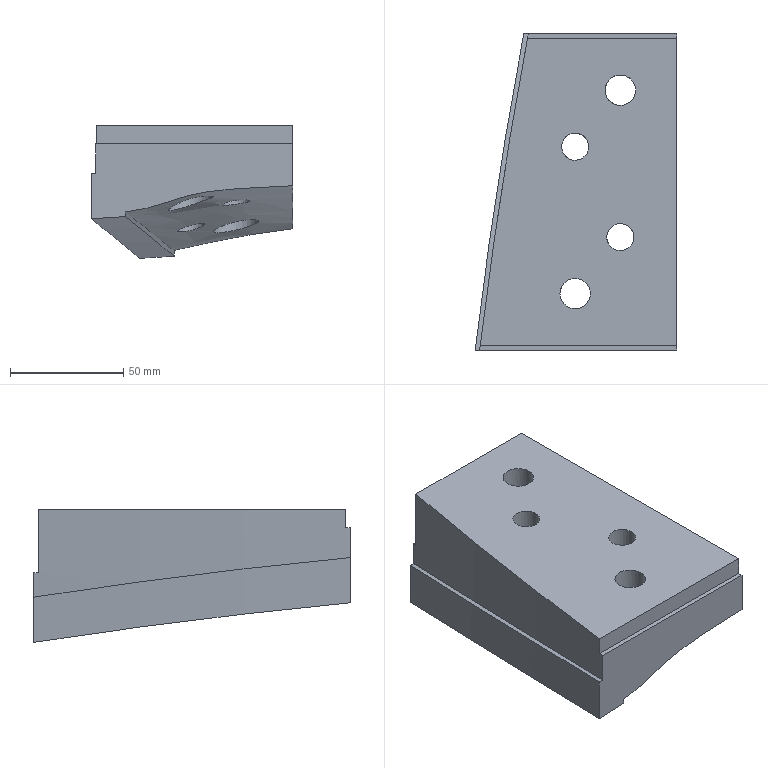Part | NX | features solid 2 | 1 solid | 22 faces | box 89.253 x 140 x 58.721 mm | volume 411184 mm3 | plane 9 | spline 7 | cylinder 6 | commonest cylinder face diameters 12 x2 13.5 x2 20 x2
STEP:
#1=CARTESIAN_POINT('',(-500.628,262.08,-55.133));
#2=VERTEX_POINT('',#1);
#3=CARTESIAN_POINT('',(-497.722,266.082,-55.166));
#4=CARTESIAN_POINT('',(-501.258,262.297,-55.273));
#5=CARTESIAN_POINT('',(-501.012,257.208,-54.545));
#6=CARTESIAN_POINT('',(-497.395,253.818,-53.31));
#7=CARTESIAN_POINT('',(-492.297,253.905,-52.638));
#8=CARTESIAN_POINT('',(-488.756,257.682,-52.752));
#9=CARTESIAN_POINT('',(-488.96,262.753,-53.541));
#10=CARTESIAN_POINT('',(-492.631,266.204,-54.446));
#11=CARTESIAN_POINT('',(-497.722,266.082,-55.166));
#12=CARTESIAN_POINT('',(-501.258,262.297,-55.273));
#13=CARTESIAN_POINT('',(-501.012,257.208,-54.545));
#14=B_SPLINE_CURVE_WITH_KNOTS('',3,(#3,#4,#5,#6,#7,#8,#9,#10,#11,#12,#13),.UNSPECIFIED.,.T.,.F.,(1,1,1,1,1,1,1,1,1,1,1,1,1,1,1),(-0.01422,-0.009479,-0.00474,0.,0.00474,0.009479,0.01422,0.01896,0.0237,0.02844,0.03318,0.03792,0.04266,0.0474,0.05214),.UNSPECIFIED.);
#15=EDGE_CURVE('',#2,#2,#14,.T.);
#16=ORIENTED_EDGE('',*,*,#15,.T.);
#17=EDGE_LOOP('',(#16));
#18=FACE_BOUND('',#17,.T.);
#19=CARTESIAN_POINT('',(-524.868,233.378,-57.001));
#20=VERTEX_POINT('',#19);
#21=CARTESIAN_POINT('',(-523.703,229.59,-56.004));
#22=CARTESIAN_POINT('',(-525.128,233.316,-57.091));
#23=CARTESIAN_POINT('',(-524.989,237.412,-57.638));
#24=CARTESIAN_POINT('',(-523.231,241.148,-57.522));
#25=CARTESIAN_POINT('',(-520.2,243.845,-56.775));
#26=CARTESIAN_POINT('',(-515.217,245.579,-55.254));
#27=CARTESIAN_POINT('',(-509.957,244.317,-53.316));
#28=CARTESIAN_POINT('',(-506.29,240.431,-52.099));
#29=CARTESIAN_POINT('',(-504.368,235.344,-51.314));
#30=CARTESIAN_POINT('',(-505.755,229.711,-50.927));
#31=CARTESIAN_POINT('',(-509.906,226.077,-51.117));
#32=CARTESIAN_POINT('',(-513.781,224.812,-51.767));
#33=CARTESIAN_POINT('',(-517.684,225.118,-53.037));
#34=CARTESIAN_POINT('',(-521.1,226.783,-54.57));
#35=CARTESIAN_POINT('',(-523.703,229.59,-56.004));
#36=CARTESIAN_POINT('',(-525.128,233.316,-57.091));
#37=CARTESIAN_POINT('',(-524.989,237.412,-57.638));
#38=B_SPLINE_CURVE_WITH_KNOTS('',3,(#21,#22,#23,#24,#25,#26,#27,#28,#29,#30,#31,#32,#33,#34,#35,#36,#37),.UNSPECIFIED.,.T.,.F.,(1,1,1,1,1,1,1,1,1,1,1,1,1,1,1,1,1,1,1,1,1),(-0.01206,-0.008041,-0.004021,0.,0.004021,0.008041,0.01206,0.01608,0.02412,0.02814,0.03216,0.04021,0.04423,0.04825,0.05227,0.05629,0.06031,0.06433,0.06835,0.07237,0.07639),.UNSPECIFIED.);
#39=EDGE_CURVE('',#20,#20,#38,.T.);
#40=ORIENTED_EDGE('',*,*,#39,.F.);
#41=EDGE_LOOP('',(#40));
#42=FACE_BOUND('',#41,.T.);
#43=CARTESIAN_POINT('',(-470.,210.,-46.611));
#44=VERTEX_POINT('',#43);
#45=CARTESIAN_POINT('',(-544.144,210.,-58.181));
#46=VERTEX_POINT('',#45);
#47=CARTESIAN_POINT('',(-470.,210.,-46.611));
#48=CARTESIAN_POINT('',(-473.142,210.,-46.734));
#49=CARTESIAN_POINT('',(-479.425,210.,-46.986));
#50=CARTESIAN_POINT('',(-488.844,210.,-47.464));
#51=CARTESIAN_POINT('',(-498.259,210.,-48.122));
#52=CARTESIAN_POINT('',(-507.638,210.,-49.048));
#53=CARTESIAN_POINT('',(-516.834,210.,-50.901));
#54=CARTESIAN_POINT('',(-525.787,210.,-54.007));
#55=CARTESIAN_POINT('',(-534.818,210.,-56.749));
#56=CARTESIAN_POINT('',(-541.02,210.,-57.77));
#57=CARTESIAN_POINT('',(-544.144,210.,-58.181));
#58=B_SPLINE_CURVE_WITH_KNOTS('',3,(#47,#48,#49,#50,#51,#52,#53,#54,#55,#56,#57),.UNSPECIFIED.,.F.,.F.,(4,1,1,1,1,1,1,1,4),(0.01237,0.0218,0.03123,0.04067,0.0501,0.05953,0.06896,0.07839,0.08783),.UNSPECIFIED.);
#59=EDGE_CURVE('',#44,#46,#58,.T.);
#60=ORIENTED_EDGE('',*,*,#59,.T.);
#61=CARTESIAN_POINT('',(-522.477,350.,-75.15));
#62=VERTEX_POINT('',#61);
#63=CARTESIAN_POINT('',(-544.144,210.,-58.181));
#64=CARTESIAN_POINT('',(-543.432,215.848,-59.019));
#65=CARTESIAN_POINT('',(-542.324,224.666,-59.797));
#66=CARTESIAN_POINT('',(-540.78,236.384,-61.12));
#67=CARTESIAN_POINT('',(-539.587,245.171,-62.09));
#68=CARTESIAN_POINT('',(-538.35,254.006,-62.555));
#69=CARTESIAN_POINT('',(-537.086,262.775,-63.591));
#70=CARTESIAN_POINT('',(-535.786,271.544,-64.601));
#71=CARTESIAN_POINT('',(-534.006,283.217,-66.034));
#72=CARTESIAN_POINT('',(-531.695,297.769,-68.007));
#73=CARTESIAN_POINT('',(-529.266,312.289,-70.077));
#74=CARTESIAN_POINT('',(-527.249,323.891,-71.737));
#75=CARTESIAN_POINT('',(-525.696,332.607,-72.823));
#76=CARTESIAN_POINT('',(-524.122,341.235,-74.542));
#77=CARTESIAN_POINT('',(-523.028,347.088,-74.878));
#78=CARTESIAN_POINT('',(-522.477,350.,-75.15));
#79=B_SPLINE_CURVE_WITH_KNOTS('',3,(#63,#64,#65,#66,#67,#68,#69,#70,#71,#72,#73,#74,#75,#76,#77,#78),.UNSPECIFIED.,.F.,.F.,(4,1,1,1,1,1,1,1,1,1,1,1,1,4),(0.1259,0.1438,0.1527,0.1616,0.1705,0.1795,0.1884,0.1973,0.2151,0.233,0.2419,0.2508,0.2597,0.2686),.UNSPECIFIED.);
#80=EDGE_CURVE('',#46,#62,#79,.T.);
#81=ORIENTED_EDGE('',*,*,#80,.T.);
#82=CARTESIAN_POINT('',(-470.,350.,-65.615));
#83=VERTEX_POINT('',#82);
#84=CARTESIAN_POINT('',(-470.,350.,-65.615));
#85=CARTESIAN_POINT('',(-478.849,350.,-66.593));
#86=CARTESIAN_POINT('',(-492.017,350.,-68.687));
#87=CARTESIAN_POINT('',(-509.435,350.,-72.287));
#88=CARTESIAN_POINT('',(-518.119,350.,-74.296));
#89=CARTESIAN_POINT('',(-522.477,350.,-75.15));
#90=B_SPLINE_CURVE_WITH_KNOTS('',3,(#84,#85,#86,#87,#88,#89),.UNSPECIFIED.,.F.,.F.,(4,1,1,4),(0.,0.02666,0.04,0.05333),.UNSPECIFIED.);
#91=EDGE_CURVE('',#83,#62,#90,.T.);
#92=ORIENTED_EDGE('',*,*,#91,.F.);
#93=CARTESIAN_POINT('',(-470.,210.,-46.611));
#94=CARTESIAN_POINT('',(-470.,212.915,-47.055));
#95=CARTESIAN_POINT('',(-470.,218.761,-47.767));
#96=CARTESIAN_POINT('',(-470.,227.581,-48.329));
#97=CARTESIAN_POINT('',(-470.,236.357,-49.332));
#98=CARTESIAN_POINT('',(-470.,245.098,-50.696));
#99=CARTESIAN_POINT('',(-470.,253.942,-51.01));
#100=CARTESIAN_POINT('',(-470.,262.68,-52.403));
#101=CARTESIAN_POINT('',(-470.,271.448,-53.491));
#102=CARTESIAN_POINT('',(-470.,283.129,-55.005));
#103=CARTESIAN_POINT('',(-470.,294.811,-56.513));
#104=CARTESIAN_POINT('',(-470.,306.491,-58.03));
#105=CARTESIAN_POINT('',(-470.,315.253,-59.159));
#106=CARTESIAN_POINT('',(-470.,324.013,-60.298));
#107=CARTESIAN_POINT('',(-470.,331.232,-61.771));
#108=CARTESIAN_POINT('',(-470.,337.094,-62.392));
#109=CARTESIAN_POINT('',(-470.,342.9,-63.373));
#110=CARTESIAN_POINT('',(-470.,347.148,-64.793));
#111=CARTESIAN_POINT('',(-470.,350.,-65.615));
#112=B_SPLINE_CURVE_WITH_KNOTS('',3,(#93,#94,#95,#96,#97,#98,#99,#100,#101,#102,#103,#104,#105,#106,#107,#108,#109,#110,#111),.UNSPECIFIED.,.F.,.F.,(4,1,1,1,1,1,1,1,1,1,1,1,1,1,1,1,4),(0.1254,0.1343,0.1431,0.152,0.1608,0.1696,0.1785,0.1873,0.1962,0.2138,0.2227,0.2315,0.2403,0.2492,0.2536,0.258,0.2669),.UNSPECIFIED.);
#113=EDGE_CURVE('',#44,#83,#112,.T.);
#114=ORIENTED_EDGE('',*,*,#113,.F.);
#115=EDGE_LOOP('',(#60,#81,#92,#114));
#116=FACE_BOUND('',#115,.T.);
#117=CARTESIAN_POINT('',(-520.662,301.985,-66.934));
#118=VERTEX_POINT('',#117);
#119=CARTESIAN_POINT('',(-517.742,306.086,-67.045));
#120=CARTESIAN_POINT('',(-521.321,302.19,-67.104));
#121=CARTESIAN_POINT('',(-520.946,297.06,-66.142));
#122=CARTESIAN_POINT('',(-517.246,293.781,-64.691));
#123=CARTESIAN_POINT('',(-512.236,293.932,-63.34));
#124=CARTESIAN_POINT('',(-508.673,297.826,-63.049));
#125=CARTESIAN_POINT('',(-509.068,302.943,-64.101));
#126=CARTESIAN_POINT('',(-512.703,306.194,-65.747));
#127=CARTESIAN_POINT('',(-517.742,306.086,-67.045));
#128=CARTESIAN_POINT('',(-521.321,302.19,-67.104));
#129=CARTESIAN_POINT('',(-520.946,297.06,-66.142));
#130=B_SPLINE_CURVE_WITH_KNOTS('',3,(#119,#120,#121,#122,#123,#124,#125,#126,#127,#128,#129),.UNSPECIFIED.,.T.,.F.,(1,1,1,1,1,1,1,1,1,1,1,1,1,1,1),(-0.01442,-0.009613,-0.004806,0.,0.004806,0.009613,0.01442,0.01923,0.02403,0.02884,0.03364,0.03845,0.04326,0.04806,0.05287),.UNSPECIFIED.);
#131=EDGE_CURVE('',#118,#118,#130,.T.);
#132=ORIENTED_EDGE('',*,*,#131,.T.);
#133=EDGE_LOOP('',(#132));
#134=FACE_BOUND('',#133,.T.);
#135=CARTESIAN_POINT('',(-485.071,326.186,-62.407));
#136=VERTEX_POINT('',#135);
#137=CARTESIAN_POINT('',(-488.149,333.648,-64.251));
#138=CARTESIAN_POINT('',(-483.99,326.362,-62.241));
#139=CARTESIAN_POINT('',(-486.314,318.019,-61.23));
#140=CARTESIAN_POINT('',(-494.001,313.958,-61.995));
#141=CARTESIAN_POINT('',(-501.898,316.427,-64.409));
#142=CARTESIAN_POINT('',(-505.271,322.343,-66.559));
#143=CARTESIAN_POINT('',(-504.897,327.749,-67.252));
#144=CARTESIAN_POINT('',(-503.038,331.396,-67.351));
#145=CARTESIAN_POINT('',(-499.902,334.024,-67.137));
#146=CARTESIAN_POINT('',(-494.738,335.605,-66.229));
#147=CARTESIAN_POINT('',(-488.149,333.648,-64.251));
#148=CARTESIAN_POINT('',(-483.99,326.362,-62.241));
#149=CARTESIAN_POINT('',(-486.314,318.019,-61.23));
#150=B_SPLINE_CURVE_WITH_KNOTS('',3,(#137,#138,#139,#140,#141,#142,#143,#144,#145,#146,#147,#148,#149),.UNSPECIFIED.,.T.,.F.,(1,1,1,1,1,1,1,1,1,1,1,1,1,1,1,1,1),(-0.01996,-0.01597,-0.007984,0.,0.007984,0.01597,0.02395,0.03194,0.03593,0.03992,0.04391,0.0479,0.05589,0.06387,0.07186,0.07984,0.08782),.UNSPECIFIED.);
#151=EDGE_CURVE('',#136,#136,#150,.T.);
#152=ORIENTED_EDGE('',*,*,#151,.F.);
#153=EDGE_LOOP('',(#152));
#154=FACE_BOUND('',#153,.T.);
#155=CARTESIAN_POINT('',(-449.856,350.,-63.928));
#156=CARTESIAN_POINT('',(-450.513,346.762,-63.155));
#157=CARTESIAN_POINT('',(-451.724,340.897,-61.568));
#158=CARTESIAN_POINT('',(-453.043,332.345,-61.292));
#159=CARTESIAN_POINT('',(-454.751,323.079,-59.482));
#160=CARTESIAN_POINT('',(-456.154,313.774,-58.463));
#161=CARTESIAN_POINT('',(-457.767,303.143,-57.153));
#162=CARTESIAN_POINT('',(-459.124,293.837,-56.036));
#163=CARTESIAN_POINT('',(-460.633,283.202,-54.741));
#164=CARTESIAN_POINT('',(-461.944,273.894,-53.558));
#165=CARTESIAN_POINT('',(-463.37,263.256,-52.318));
#166=CARTESIAN_POINT('',(-464.678,253.944,-50.886));
#167=CARTESIAN_POINT('',(-465.814,243.308,-50.34));
#168=CARTESIAN_POINT('',(-467.008,233.989,-48.769));
#169=CARTESIAN_POINT('',(-468.149,223.335,-47.963));
#170=CARTESIAN_POINT('',(-468.958,215.772,-47.418));
#171=CARTESIAN_POINT('',(-469.452,210.889,-46.724));
#172=CARTESIAN_POINT('',(-469.542,210.,-46.593));
#173=CARTESIAN_POINT('',(-458.824,350.,-64.479));
#174=CARTESIAN_POINT('',(-459.498,346.762,-63.609));
#175=CARTESIAN_POINT('',(-460.741,340.897,-61.784));
#176=CARTESIAN_POINT('',(-462.105,332.345,-61.543));
#177=CARTESIAN_POINT('',(-463.848,323.079,-59.715));
#178=CARTESIAN_POINT('',(-465.277,313.774,-58.704));
#179=CARTESIAN_POINT('',(-466.92,303.143,-57.386));
#180=CARTESIAN_POINT('',(-468.301,293.837,-56.271));
#181=CARTESIAN_POINT('',(-469.838,283.202,-54.976));
#182=CARTESIAN_POINT('',(-471.174,273.894,-53.77));
#183=CARTESIAN_POINT('',(-472.622,263.256,-52.566));
#184=CARTESIAN_POINT('',(-473.97,253.944,-51.01));
#185=CARTESIAN_POINT('',(-475.086,243.308,-50.852));
#186=CARTESIAN_POINT('',(-476.315,233.989,-49.173));
#187=CARTESIAN_POINT('',(-477.474,223.335,-48.448));
#188=CARTESIAN_POINT('',(-478.287,215.772,-47.966));
#189=CARTESIAN_POINT('',(-478.816,210.889,-47.117));
#190=CARTESIAN_POINT('',(-478.912,210.,-46.959));
#191=CARTESIAN_POINT('',(-473.435,350.,-65.726));
#192=CARTESIAN_POINT('',(-474.128,346.762,-64.77));
#193=CARTESIAN_POINT('',(-475.402,340.897,-62.756));
#194=CARTESIAN_POINT('',(-476.899,332.345,-62.044));
#195=CARTESIAN_POINT('',(-478.685,323.079,-60.267));
#196=CARTESIAN_POINT('',(-480.159,313.774,-59.241));
#197=CARTESIAN_POINT('',(-481.852,303.143,-57.9));
#198=CARTESIAN_POINT('',(-483.273,293.837,-56.782));
#199=CARTESIAN_POINT('',(-484.856,283.202,-55.473));
#200=CARTESIAN_POINT('',(-486.235,273.894,-54.23));
#201=CARTESIAN_POINT('',(-487.725,263.256,-53.066));
#202=CARTESIAN_POINT('',(-489.113,253.944,-51.363));
#203=CARTESIAN_POINT('',(-490.278,243.308,-51.691));
#204=CARTESIAN_POINT('',(-491.533,233.989,-49.951));
#205=CARTESIAN_POINT('',(-492.732,223.335,-49.263));
#206=CARTESIAN_POINT('',(-493.563,215.772,-48.871));
#207=CARTESIAN_POINT('',(-494.125,210.889,-47.791));
#208=CARTESIAN_POINT('',(-494.227,210.,-47.592));
#209=CARTESIAN_POINT('',(-493.528,350.,-69.004));
#210=CARTESIAN_POINT('',(-494.177,346.762,-68.601));
#211=CARTESIAN_POINT('',(-495.352,340.897,-67.906));
#212=CARTESIAN_POINT('',(-496.974,332.345,-65.437));
#213=CARTESIAN_POINT('',(-498.685,323.079,-64.394));
#214=CARTESIAN_POINT('',(-500.264,313.774,-63.172));
#215=CARTESIAN_POINT('',(-502.032,303.143,-61.81));
#216=CARTESIAN_POINT('',(-503.541,293.837,-60.561));
#217=CARTESIAN_POINT('',(-505.215,283.202,-59.125));
#218=CARTESIAN_POINT('',(-506.619,273.894,-57.989));
#219=CARTESIAN_POINT('',(-508.284,263.256,-56.294));
#220=CARTESIAN_POINT('',(-509.365,253.944,-56.111));
#221=CARTESIAN_POINT('',(-511.739,243.308,-51.7));
#222=CARTESIAN_POINT('',(-512.661,233.989,-51.783));
#223=CARTESIAN_POINT('',(-513.992,223.335,-50.536));
#224=CARTESIAN_POINT('',(-515.05,215.772,-49.254));
#225=CARTESIAN_POINT('',(-515.27,210.889,-49.774));
#226=CARTESIAN_POINT('',(-515.308,210.,-49.876));
#227=CARTESIAN_POINT('',(-508.923,350.,-72.168));
#228=CARTESIAN_POINT('',(-509.556,346.762,-72.055));
#229=CARTESIAN_POINT('',(-510.683,340.897,-72.06));
#230=CARTESIAN_POINT('',(-512.084,332.345,-70.049));
#231=CARTESIAN_POINT('',(-513.723,323.079,-69.619));
#232=CARTESIAN_POINT('',(-515.396,313.774,-68.202));
#233=CARTESIAN_POINT('',(-517.233,303.143,-66.813));
#234=CARTESIAN_POINT('',(-518.821,293.837,-65.444));
#235=CARTESIAN_POINT('',(-520.563,283.202,-63.955));
#236=CARTESIAN_POINT('',(-522.016,273.894,-62.801));
#237=CARTESIAN_POINT('',(-523.686,263.256,-61.26));
#238=CARTESIAN_POINT('',(-525.022,253.944,-60.29));
#239=CARTESIAN_POINT('',(-526.333,243.308,-59.951));
#240=CARTESIAN_POINT('',(-527.611,233.989,-58.843));
#241=CARTESIAN_POINT('',(-529.001,223.335,-57.605));
#242=CARTESIAN_POINT('',(-529.929,215.772,-56.934));
#243=CARTESIAN_POINT('',(-530.518,210.889,-56.17));
#244=CARTESIAN_POINT('',(-530.626,210.,-56.028));
#245=CARTESIAN_POINT('',(-518.692,350.,-74.418));
#246=CARTESIAN_POINT('',(-519.336,346.762,-74.182));
#247=CARTESIAN_POINT('',(-520.478,340.897,-73.967));
#248=CARTESIAN_POINT('',(-521.951,332.345,-72.164));
#249=CARTESIAN_POINT('',(-523.639,323.079,-71.205));
#250=CARTESIAN_POINT('',(-525.351,313.774,-69.84));
#251=CARTESIAN_POINT('',(-527.235,303.143,-68.345));
#252=CARTESIAN_POINT('',(-528.845,293.837,-67.064));
#253=CARTESIAN_POINT('',(-530.615,283.202,-65.615));
#254=CARTESIAN_POINT('',(-532.096,273.894,-64.454));
#255=CARTESIAN_POINT('',(-533.76,263.256,-63.183));
#256=CARTESIAN_POINT('',(-535.149,253.944,-62.094));
#257=CARTESIAN_POINT('',(-536.435,243.308,-61.647));
#258=CARTESIAN_POINT('',(-537.767,233.989,-60.473));
#259=CARTESIAN_POINT('',(-539.173,223.335,-59.346));
#260=CARTESIAN_POINT('',(-540.107,215.772,-58.653));
#261=CARTESIAN_POINT('',(-540.738,210.889,-57.918));
#262=CARTESIAN_POINT('',(-540.853,210.,-57.782));
#263=CARTESIAN_POINT('',(-522.907,350.,-75.234));
#264=CARTESIAN_POINT('',(-523.558,346.762,-74.932));
#265=CARTESIAN_POINT('',(-524.71,340.897,-74.582));
#266=CARTESIAN_POINT('',(-526.228,332.345,-72.867));
#267=CARTESIAN_POINT('',(-527.941,323.079,-71.701));
#268=CARTESIAN_POINT('',(-529.668,313.774,-70.369));
#269=CARTESIAN_POINT('',(-531.571,303.143,-68.846));
#270=CARTESIAN_POINT('',(-533.189,293.837,-67.602));
#271=CARTESIAN_POINT('',(-534.971,283.202,-66.172));
#272=CARTESIAN_POINT('',(-536.463,273.894,-65.007));
#273=CARTESIAN_POINT('',(-538.128,263.256,-63.818));
#274=CARTESIAN_POINT('',(-539.531,253.944,-62.697));
#275=CARTESIAN_POINT('',(-540.854,243.308,-62.069));
#276=CARTESIAN_POINT('',(-542.194,233.989,-60.923));
#277=CARTESIAN_POINT('',(-543.607,223.335,-59.841));
#278=CARTESIAN_POINT('',(-544.55,215.772,-59.117));
#279=CARTESIAN_POINT('',(-545.183,210.889,-58.451));
#280=CARTESIAN_POINT('',(-545.298,210.,-58.327));
#281=B_SPLINE_SURFACE_WITH_KNOTS('',3,3,((#155,#156,#157,#158,#159,#160,#161,#162,#163,#164,#165,#166,#167,#168,#169,#170,#171,#172),(#173,#174,#175,#176,#177,#178,#179,#180,#181,#182,#183,#184,#185,#186,#187,#188,#189,#190),(#191,#192,#193,#194,#195,#196,#197,#198,#199,#200,#201,#202,#203,#204,#205,#206,#207,#208),(#209,#210,#211,#212,#213,#214,#215,#216,#217,#218,#219,#220,#221,#222,#223,#224,#225,#226),(#227,#228,#229,#230,#231,#232,#233,#234,#235,#236,#237,#238,#239,#240,#241,#242,#243,#244),(#245,#246,#247,#248,#249,#250,#251,#252,#253,#254,#255,#256,#257,#258,#259,#260,#261,#262),(#263,#264,#265,#266,#267,#268,#269,#270,#271,#272,#273,#274,#275,#276,#277,#278,#279,#280)),.UNSPECIFIED.,.F.,.F.,.F.,(4,1,1,1,4),(4,1,1,1,1,1,1,1,1,1,1,1,1,1,1,4),(0.9128,0.9375,0.9531,0.9688,0.9806),(0.2465,0.2656,0.2812,0.2969,0.3203,0.3359,0.3594,0.375,0.3984,0.4141,0.4375,0.4531,0.4766,0.4922,0.5156,0.5208),.UNSPECIFIED.);
#282=ADVANCED_FACE('',(#18,#42,#116,#134,#154),#281,.F.);
#283=CARTESIAN_POINT('',(-470.,348.,-48.));
#284=VERTEX_POINT('',#283);
#285=CARTESIAN_POINT('',(-536.081,348.,-48.));
#286=VERTEX_POINT('',#285);
#287=CARTESIAN_POINT('',(-470.,348.,-48.));
#288=DIRECTION('',(1.,0.,0.));
#289=VECTOR('',#288,1000.);
#290=LINE('',#287,#289);
#291=EDGE_CURVE('',#284,#286,#290,.F.);
#292=ORIENTED_EDGE('',*,*,#291,.F.);
#293=CARTESIAN_POINT('',(-470.,350.,-48.));
#294=VERTEX_POINT('',#293);
#295=CARTESIAN_POINT('',(-470.,350.,-48.));
#296=DIRECTION('',(0.,1.,0.));
#297=VECTOR('',#296,1000.);
#298=LINE('',#295,#297);
#299=EDGE_CURVE('',#294,#284,#298,.F.);
#300=ORIENTED_EDGE('',*,*,#299,.F.);
#301=CARTESIAN_POINT('',(-535.705,350.,-48.));
#302=VERTEX_POINT('',#301);
#303=CARTESIAN_POINT('',(-470.,350.,-48.));
#304=DIRECTION('',(1.,0.,0.));
#305=VECTOR('',#304,1000.);
#306=LINE('',#303,#305);
#307=EDGE_CURVE('',#294,#302,#306,.F.);
#308=ORIENTED_EDGE('',*,*,#307,.T.);
#309=CARTESIAN_POINT('',(-536.081,348.,-48.));
#310=CARTESIAN_POINT('',(-535.956,348.667,-48.));
#311=CARTESIAN_POINT('',(-535.831,349.333,-48.));
#312=CARTESIAN_POINT('',(-535.705,350.,-48.));
#313=B_SPLINE_CURVE_WITH_KNOTS('',3,(#309,#310,#311,#312),.UNSPECIFIED.,.F.,.F.,(4,4),(0.01222,0.01426),.UNSPECIFIED.);
#314=EDGE_CURVE('',#302,#286,#313,.F.);
#315=ORIENTED_EDGE('',*,*,#314,.T.);
#316=EDGE_LOOP('',(#292,#300,#308,#315));
#317=FACE_BOUND('',#316,.T.);
#318=CARTESIAN_POINT('',(-470.,350.,-48.));
#319=DIRECTION('',(0.,0.,1.));
#320=DIRECTION('',(1.,0.,0.));
#321=AXIS2_PLACEMENT_3D('',#318,#319,#320);
#322=PLANE('',#321);
#323=ADVANCED_FACE('',(#317),#322,.T.);
#324=CARTESIAN_POINT('',(-535.705,350.,-58.778));
#325=VERTEX_POINT('',#324);
#326=CARTESIAN_POINT('',(-535.705,350.,-23.36));
#327=DIRECTION('',(0.,0.,1.));
#328=VECTOR('',#327,1000.);
#329=LINE('',#326,#328);
#330=EDGE_CURVE('',#325,#302,#329,.T.);
#331=ORIENTED_EDGE('',*,*,#330,.T.);
#332=ORIENTED_EDGE('',*,*,#307,.F.);
#333=CARTESIAN_POINT('',(-470.,350.,-40.306));
#334=DIRECTION('',(0.,0.,-1.));
#335=VECTOR('',#334,1000.);
#336=LINE('',#333,#335);
#337=EDGE_CURVE('',#83,#294,#336,.F.);
#338=ORIENTED_EDGE('',*,*,#337,.F.);
#339=ORIENTED_EDGE('',*,*,#91,.T.);
#340=CARTESIAN_POINT('',(-522.477,350.,-77.768));
#341=VERTEX_POINT('',#340);
#342=CARTESIAN_POINT('',(-522.477,350.,-46.));
#343=DIRECTION('',(0.,0.,1.));
#344=VECTOR('',#343,1000.);
#345=LINE('',#342,#344);
#346=EDGE_CURVE('',#341,#62,#345,.T.);
#347=ORIENTED_EDGE('',*,*,#346,.F.);
#348=CARTESIAN_POINT('',(-537.74,350.,-78.721));
#349=VERTEX_POINT('',#348);
#350=CARTESIAN_POINT('',(-537.74,350.,-78.721));
#351=CARTESIAN_POINT('',(-532.653,350.,-78.396));
#352=CARTESIAN_POINT('',(-527.565,350.,-78.079));
#353=CARTESIAN_POINT('',(-522.477,350.,-77.768));
#354=B_SPLINE_CURVE_WITH_KNOTS('',3,(#350,#351,#352,#353),.UNSPECIFIED.,.F.,.F.,(4,4),(0.03478,0.05008),.UNSPECIFIED.);
#355=EDGE_CURVE('',#349,#341,#354,.T.);
#356=ORIENTED_EDGE('',*,*,#355,.F.);
#357=CARTESIAN_POINT('',(-537.74,350.,-58.721));
#358=VERTEX_POINT('',#357);
#359=CARTESIAN_POINT('',(-537.74,350.,-41.428));
#360=DIRECTION('',(0.,0.,1.));
#361=VECTOR('',#360,1000.);
#362=LINE('',#359,#361);
#363=EDGE_CURVE('',#358,#349,#362,.F.);
#364=ORIENTED_EDGE('',*,*,#363,.F.);
#365=CARTESIAN_POINT('',(-535.705,350.,-58.778));
#366=CARTESIAN_POINT('',(-536.384,350.,-58.759));
#367=CARTESIAN_POINT('',(-537.062,350.,-58.74));
#368=CARTESIAN_POINT('',(-537.74,350.,-58.721));
#369=B_SPLINE_CURVE_WITH_KNOTS('',3,(#365,#366,#367,#368),.UNSPECIFIED.,.F.,.F.,(4,4),(0.008143,0.01018),.UNSPECIFIED.);
#370=EDGE_CURVE('',#358,#325,#369,.F.);
#371=ORIENTED_EDGE('',*,*,#370,.T.);
#372=EDGE_LOOP('',(#331,#332,#338,#339,#347,#356,#364,#371));
#373=FACE_BOUND('',#372,.T.);
#374=CARTESIAN_POINT('',(440.921,350.,-40.306));
#375=DIRECTION('',(0.,1.,0.));
#376=DIRECTION('',(0.,0.,1.));
#377=AXIS2_PLACEMENT_3D('',#374,#375,#376);
#378=PLANE('',#377);
#379=ADVANCED_FACE('',(#373),#378,.T.);
#380=CARTESIAN_POINT('',(-470.,348.,-20.));
#381=VERTEX_POINT('',#380);
#382=CARTESIAN_POINT('',(-470.,348.,12.));
#383=DIRECTION('',(0.,0.,1.));
#384=VECTOR('',#383,1000.);
#385=LINE('',#382,#384);
#386=EDGE_CURVE('',#381,#284,#385,.F.);
#387=ORIENTED_EDGE('',*,*,#386,.T.);
#388=ORIENTED_EDGE('',*,*,#291,.T.);
#389=CARTESIAN_POINT('',(-536.081,348.,-20.));
#390=VERTEX_POINT('',#389);
#391=CARTESIAN_POINT('',(-536.081,348.,-18.));
#392=DIRECTION('',(0.,0.,1.));
#393=VECTOR('',#392,1000.);
#394=LINE('',#391,#393);
#395=EDGE_CURVE('',#390,#286,#394,.F.);
#396=ORIENTED_EDGE('',*,*,#395,.F.);
#397=CARTESIAN_POINT('',(-470.,348.,-20.));
#398=DIRECTION('',(-1.,0.,0.));
#399=VECTOR('',#398,1000.);
#400=LINE('',#397,#399);
#401=EDGE_CURVE('',#381,#390,#400,.T.);
#402=ORIENTED_EDGE('',*,*,#401,.F.);
#403=EDGE_LOOP('',(#387,#388,#396,#402));
#404=FACE_BOUND('',#403,.T.);
#405=CARTESIAN_POINT('',(-470.,348.,12.));
#406=DIRECTION('',(0.,1.,0.));
#407=DIRECTION('',(-1.,0.,0.));
#408=AXIS2_PLACEMENT_3D('',#405,#406,#407);
#409=PLANE('',#408);
#410=ADVANCED_FACE('',(#404),#409,.T.);
#411=CARTESIAN_POINT('',(-544.144,210.,-60.227));
#412=VERTEX_POINT('',#411);
#413=CARTESIAN_POINT('',(-544.144,210.,-60.227));
#414=CARTESIAN_POINT('',(-538.417,257.027,-64.777));
#415=CARTESIAN_POINT('',(-531.226,303.745,-70.657));
#416=CARTESIAN_POINT('',(-522.477,350.,-77.768));
#417=B_SPLINE_CURVE_WITH_KNOTS('',3,(#413,#414,#415,#416),.UNSPECIFIED.,.F.,.F.,(4,4),(0.1259,0.2687),.UNSPECIFIED.);
#418=EDGE_CURVE('',#412,#341,#417,.T.);
#419=ORIENTED_EDGE('',*,*,#418,.T.);
#420=ORIENTED_EDGE('',*,*,#346,.T.);
#421=ORIENTED_EDGE('',*,*,#80,.F.);
#422=CARTESIAN_POINT('',(-544.144,210.,-63.127));
#423=DIRECTION('',(0.,0.,1.));
#424=VECTOR('',#423,1000.);
#425=LINE('',#422,#424);
#426=EDGE_CURVE('',#412,#46,#425,.T.);
#427=ORIENTED_EDGE('',*,*,#426,.F.);
#428=EDGE_LOOP('',(#419,#420,#421,#427));
#429=FACE_BOUND('',#428,.T.);
#430=CARTESIAN_POINT('',(-522.477,350.,-77.886));
#431=CARTESIAN_POINT('',(-522.477,350.,-58.063));
#432=CARTESIAN_POINT('',(-524.645,338.539,-77.886));
#433=CARTESIAN_POINT('',(-524.645,338.539,-58.063));
#434=CARTESIAN_POINT('',(-528.8,315.507,-77.886));
#435=CARTESIAN_POINT('',(-528.8,315.507,-58.063));
#436=CARTESIAN_POINT('',(-534.491,280.641,-77.886));
#437=CARTESIAN_POINT('',(-534.491,280.641,-58.063));
#438=CARTESIAN_POINT('',(-538.785,251.287,-77.886));
#439=CARTESIAN_POINT('',(-538.785,251.287,-58.063));
#440=CARTESIAN_POINT('',(-541.548,230.648,-77.886));
#441=CARTESIAN_POINT('',(-541.548,230.648,-58.063));
#442=CARTESIAN_POINT('',(-543.069,218.732,-77.886));
#443=CARTESIAN_POINT('',(-543.069,218.732,-58.063));
#444=CARTESIAN_POINT('',(-543.788,212.925,-77.886));
#445=CARTESIAN_POINT('',(-543.788,212.925,-58.063));
#446=CARTESIAN_POINT('',(-544.144,210.,-77.886));
#447=CARTESIAN_POINT('',(-544.144,210.,-58.063));
#448=B_SPLINE_SURFACE_WITH_KNOTS('',3,1,((#430,#431),(#432,#433),(#434,#435),(#436,#437),(#438,#439),(#440,#441),(#442,#443),(#444,#445),(#446,#447)),.SURF_OF_LINEAR_EXTRUSION.,.F.,.F.,.F.,(4,1,1,1,1,1,4),(2,2),(0.005019,0.1372,0.2694,0.4015,0.4676,0.5007,0.5337),(0.,1.),.UNSPECIFIED.);
#449=ADVANCED_FACE('',(#429),#448,.F.);
#450=CARTESIAN_POINT('',(-557.238,210.,-41.223));
#451=VERTEX_POINT('',#450);
#452=CARTESIAN_POINT('',(-557.238,210.,-41.223));
#453=CARTESIAN_POINT('',(-551.535,257.074,-45.781));
#454=CARTESIAN_POINT('',(-544.405,303.746,-51.67));
#455=CARTESIAN_POINT('',(-535.705,350.,-58.778));
#456=B_SPLINE_CURVE_WITH_KNOTS('',3,(#452,#453,#454,#455),.UNSPECIFIED.,.F.,.F.,(4,4),(0.4694,1.001),.UNSPECIFIED.);
#457=EDGE_CURVE('',#325,#451,#456,.F.);
#458=ORIENTED_EDGE('',*,*,#457,.F.);
#459=ORIENTED_EDGE('',*,*,#370,.F.);
#460=CARTESIAN_POINT('',(-559.253,210.,-41.2));
#461=VERTEX_POINT('',#460);
#462=CARTESIAN_POINT('',(-537.74,350.,-58.721));
#463=CARTESIAN_POINT('',(-539.944,338.283,-56.922));
#464=CARTESIAN_POINT('',(-544.14,314.869,-53.494));
#465=CARTESIAN_POINT('',(-549.8,279.843,-48.863));
#466=CARTESIAN_POINT('',(-554.857,244.877,-44.737));
#467=CARTESIAN_POINT('',(-557.83,221.759,-42.336));
#468=CARTESIAN_POINT('',(-559.253,210.,-41.2));
#469=B_SPLINE_CURVE_WITH_KNOTS('',3,(#462,#463,#464,#465,#466,#467,#468),.UNSPECIFIED.,.F.,.F.,(4,1,1,1,4),(0.,0.1328,0.2657,0.3985,0.5314),.UNSPECIFIED.);
#470=EDGE_CURVE('',#358,#461,#469,.T.);
#471=ORIENTED_EDGE('',*,*,#470,.T.);
#472=CARTESIAN_POINT('',(-557.238,210.,-41.223));
#473=CARTESIAN_POINT('',(-557.91,210.,-41.215));
#474=CARTESIAN_POINT('',(-558.581,210.,-41.208));
#475=CARTESIAN_POINT('',(-559.253,210.,-41.2));
#476=B_SPLINE_CURVE_WITH_KNOTS('',3,(#472,#473,#474,#475),.UNSPECIFIED.,.F.,.F.,(4,4),(0.,0.002015),.UNSPECIFIED.);
#477=EDGE_CURVE('',#451,#461,#476,.T.);
#478=ORIENTED_EDGE('',*,*,#477,.F.);
#479=EDGE_LOOP('',(#458,#459,#471,#478));
#480=FACE_BOUND('',#479,.T.);
#481=CARTESIAN_POINT('',(-535.549,350.834,-58.906));
#482=CARTESIAN_POINT('',(-535.624,350.433,-58.844));
#483=CARTESIAN_POINT('',(-535.699,350.032,-58.782));
#484=CARTESIAN_POINT('',(-535.775,349.63,-58.721));
#485=CARTESIAN_POINT('',(-543.951,306.163,-52.041));
#486=CARTESIAN_POINT('',(-550.731,262.328,-46.45));
#487=CARTESIAN_POINT('',(-556.622,215.058,-41.716));
#488=CARTESIAN_POINT('',(-556.999,211.985,-41.414));
#489=CARTESIAN_POINT('',(-557.37,208.911,-41.118));
#490=CARTESIAN_POINT('',(-537.514,351.205,-58.906));
#491=CARTESIAN_POINT('',(-537.589,350.803,-58.844));
#492=CARTESIAN_POINT('',(-537.665,350.402,-58.782));
#493=CARTESIAN_POINT('',(-537.74,350.,-58.721));
#494=CARTESIAN_POINT('',(-545.924,306.491,-52.041));
#495=CARTESIAN_POINT('',(-552.711,262.613,-46.45));
#496=CARTESIAN_POINT('',(-558.607,215.302,-41.716));
#497=CARTESIAN_POINT('',(-558.984,212.227,-41.414));
#498=CARTESIAN_POINT('',(-559.356,209.15,-41.118));
#499=B_SPLINE_SURFACE_WITH_KNOTS('',1,3,((#481,#482,#483,#484,#485,#486,#487,#488,#489),(#490,#491,#492,#493,#494,#495,#496,#497,#498)),.RULED_SURF.,.F.,.F.,.F.,(2,2),(4,3,2,4),(0.,1.),(-0.004615,0.,0.5,0.5347),.UNSPECIFIED.);
#500=ADVANCED_FACE('',(#480),#499,.T.);
#501=ORIENTED_EDGE('',*,*,#470,.F.);
#502=ORIENTED_EDGE('',*,*,#363,.T.);
#503=CARTESIAN_POINT('',(-559.253,210.,-61.2));
#504=VERTEX_POINT('',#503);
#505=CARTESIAN_POINT('',(-537.74,350.,-78.721));
#506=CARTESIAN_POINT('',(-546.44,303.747,-71.62));
#507=CARTESIAN_POINT('',(-553.557,257.075,-65.75));
#508=CARTESIAN_POINT('',(-559.253,210.,-61.2));
#509=B_SPLINE_CURVE_WITH_KNOTS('',3,(#505,#506,#507,#508),.UNSPECIFIED.,.F.,.F.,(4,4),(0.3116,0.4563),.UNSPECIFIED.);
#510=EDGE_CURVE('',#349,#504,#509,.T.);
#511=ORIENTED_EDGE('',*,*,#510,.T.);
#512=CARTESIAN_POINT('',(-559.253,210.,-55.491));
#513=DIRECTION('',(0.,0.,1.));
#514=VECTOR('',#513,1000.);
#515=LINE('',#512,#514);
#516=EDGE_CURVE('',#461,#504,#515,.F.);
#517=ORIENTED_EDGE('',*,*,#516,.F.);
#518=EDGE_LOOP('',(#501,#502,#511,#517));
#519=FACE_BOUND('',#518,.T.);
#520=CARTESIAN_POINT('',(-559.355,209.153,-78.946));
#521=CARTESIAN_POINT('',(-559.355,209.153,-40.975));
#522=CARTESIAN_POINT('',(-553.648,256.468,-78.946));
#523=CARTESIAN_POINT('',(-553.648,256.468,-40.975));
#524=CARTESIAN_POINT('',(-546.491,303.477,-78.946));
#525=CARTESIAN_POINT('',(-546.491,303.477,-40.975));
#526=CARTESIAN_POINT('',(-537.74,350.,-78.946));
#527=CARTESIAN_POINT('',(-537.74,350.,-40.975));
#528=B_SPLINE_SURFACE_WITH_KNOTS('',3,1,((#520,#521),(#522,#523),(#524,#525),(#526,#527)),.SURF_OF_LINEAR_EXTRUSION.,.F.,.F.,.F.,(4,4),(2,2),(0.3283,0.4272),(0.,1.),.PIECEWISE_BEZIER_KNOTS.);
#529=ADVANCED_FACE('',(#519),#528,.F.);
#530=ORIENTED_EDGE('',*,*,#510,.F.);
#531=ORIENTED_EDGE('',*,*,#355,.T.);
#532=ORIENTED_EDGE('',*,*,#418,.F.);
#533=CARTESIAN_POINT('',(-559.253,210.,-61.2));
#534=CARTESIAN_POINT('',(-554.217,210.,-60.868));
#535=CARTESIAN_POINT('',(-549.18,210.,-60.544));
#536=CARTESIAN_POINT('',(-544.144,210.,-60.227));
#537=B_SPLINE_CURVE_WITH_KNOTS('',3,(#533,#534,#535,#536),.UNSPECIFIED.,.F.,.F.,(4,4),(0.01195,0.02709),.UNSPECIFIED.);
#538=EDGE_CURVE('',#504,#412,#537,.T.);
#539=ORIENTED_EDGE('',*,*,#538,.F.);
#540=EDGE_LOOP('',(#530,#531,#532,#539));
#541=FACE_BOUND('',#540,.T.);
#542=CARTESIAN_POINT('',(-559.416,351.134,-80.335));
#543=CARTESIAN_POINT('',(-547.03,351.032,-79.478));
#544=CARTESIAN_POINT('',(-534.643,350.935,-78.665));
#545=CARTESIAN_POINT('',(-522.256,350.843,-77.894));
#546=CARTESIAN_POINT('',(-559.434,303.646,-72.44));
#547=CARTESIAN_POINT('',(-547.048,303.545,-71.593));
#548=CARTESIAN_POINT('',(-534.662,303.45,-70.792));
#549=CARTESIAN_POINT('',(-522.275,303.359,-70.032));
#550=CARTESIAN_POINT('',(-559.453,256.323,-66.037));
#551=CARTESIAN_POINT('',(-547.068,256.223,-65.201));
#552=CARTESIAN_POINT('',(-534.682,256.128,-64.41));
#553=CARTESIAN_POINT('',(-522.294,256.039,-63.66));
#554=CARTESIAN_POINT('',(-559.473,209.163,-61.127));
#555=CARTESIAN_POINT('',(-547.088,209.064,-60.301));
#556=CARTESIAN_POINT('',(-534.701,208.971,-59.52));
#557=CARTESIAN_POINT('',(-522.314,208.883,-58.779));
#558=B_SPLINE_SURFACE_WITH_KNOTS('',3,3,((#542,#543,#544,#545),(#546,#547,#548,#549),(#550,#551,#552,#553),(#554,#555,#556,#557)),.UNSPECIFIED.,.F.,.F.,.F.,(4,4),(4,4),(0.3051,0.5209),(0.1181,0.1635),.UNSPECIFIED.);
#559=ADVANCED_FACE('',(#541),#558,.F.);
#560=CARTESIAN_POINT('',(-489.,260.,-20.));
#561=VERTEX_POINT('',#560);
#562=CARTESIAN_POINT('',(-495.,260.,-20.));
#563=DIRECTION('',(0.,0.,1.));
#564=DIRECTION('',(1.,0.,0.));
#565=AXIS2_PLACEMENT_3D('',#562,#563,#564);
#566=CIRCLE('',#565,6.);
#567=EDGE_CURVE('',#561,#561,#566,.F.);
#568=ORIENTED_EDGE('',*,*,#567,.T.);
#569=EDGE_LOOP('',(#568));
#570=FACE_BOUND('',#569,.T.);
#571=CARTESIAN_POINT('',(-501.75,325.,-20.));
#572=VERTEX_POINT('',#571);
#573=CARTESIAN_POINT('',(-495.,325.,-20.));
#574=DIRECTION('',(0.,0.,-1.));
#575=DIRECTION('',(-1.,0.,0.));
#576=AXIS2_PLACEMENT_3D('',#573,#574,#575);
#577=CIRCLE('',#576,6.75);
#578=EDGE_CURVE('',#572,#572,#577,.T.);
#579=ORIENTED_EDGE('',*,*,#578,.T.);
#580=EDGE_LOOP('',(#579));
#581=FACE_BOUND('',#580,.T.);
#582=CARTESIAN_POINT('',(-509.,300.,-20.));
#583=VERTEX_POINT('',#582);
#584=CARTESIAN_POINT('',(-515.,300.,-20.));
#585=DIRECTION('',(0.,0.,1.));
#586=DIRECTION('',(1.,0.,0.));
#587=AXIS2_PLACEMENT_3D('',#584,#585,#586);
#588=CIRCLE('',#587,6.);
#589=EDGE_CURVE('',#583,#583,#588,.F.);
#590=ORIENTED_EDGE('',*,*,#589,.T.);
#591=EDGE_LOOP('',(#590));
#592=FACE_BOUND('',#591,.T.);
#593=CARTESIAN_POINT('',(-521.75,235.,-20.));
#594=VERTEX_POINT('',#593);
#595=CARTESIAN_POINT('',(-515.,235.,-20.));
#596=DIRECTION('',(0.,0.,-1.));
#597=DIRECTION('',(-1.,0.,0.));
#598=AXIS2_PLACEMENT_3D('',#595,#596,#597);
#599=CIRCLE('',#598,6.75);
#600=EDGE_CURVE('',#594,#594,#599,.T.);
#601=ORIENTED_EDGE('',*,*,#600,.T.);
#602=EDGE_LOOP('',(#601));
#603=FACE_BOUND('',#602,.T.);
#604=CARTESIAN_POINT('',(-556.995,212.,-20.));
#605=VERTEX_POINT('',#604);
#606=CARTESIAN_POINT('',(-470.,212.,-20.));
#607=VERTEX_POINT('',#606);
#608=CARTESIAN_POINT('',(0.,212.,-20.));
#609=DIRECTION('',(-1.,0.,0.));
#610=VECTOR('',#609,1000.);
#611=LINE('',#608,#610);
#612=EDGE_CURVE('',#605,#607,#611,.F.);
#613=ORIENTED_EDGE('',*,*,#612,.T.);
#614=CARTESIAN_POINT('',(-470.,348.,-20.));
#615=CARTESIAN_POINT('',(-470.,302.667,-20.));
#616=CARTESIAN_POINT('',(-470.,257.333,-20.));
#617=CARTESIAN_POINT('',(-470.,212.,-20.));
#618=B_SPLINE_CURVE_WITH_KNOTS('',3,(#614,#615,#616,#617),.UNSPECIFIED.,.F.,.F.,(4,4),(0.,1.),.UNSPECIFIED.);
#619=EDGE_CURVE('',#607,#381,#618,.F.);
#620=ORIENTED_EDGE('',*,*,#619,.T.);
#621=ORIENTED_EDGE('',*,*,#401,.T.);
#622=CARTESIAN_POINT('',(-556.995,212.,-20.));
#623=CARTESIAN_POINT('',(-551.326,258.485,-20.));
#624=CARTESIAN_POINT('',(-544.355,303.818,-20.));
#625=CARTESIAN_POINT('',(-536.081,348.,-20.));
#626=B_SPLINE_CURVE_WITH_KNOTS('',3,(#622,#623,#624,#625),.UNSPECIFIED.,.F.,.F.,(4,4),(0.,1.),.UNSPECIFIED.);
#627=EDGE_CURVE('',#605,#390,#626,.T.);
#628=ORIENTED_EDGE('',*,*,#627,.F.);
#629=EDGE_LOOP('',(#613,#620,#621,#628));
#630=FACE_BOUND('',#629,.T.);
#631=CARTESIAN_POINT('',(0.,0.,-20.));
#632=DIRECTION('',(0.,0.,1.));
#633=DIRECTION('',(-1.,0.,0.));
#634=AXIS2_PLACEMENT_3D('',#631,#632,#633);
#635=PLANE('',#634);
#636=ADVANCED_FACE('',(#570,#581,#592,#603,#630),#635,.T.);
#637=ORIENTED_EDGE('',*,*,#627,.T.);
#638=ORIENTED_EDGE('',*,*,#395,.T.);
#639=ORIENTED_EDGE('',*,*,#314,.F.);
#640=ORIENTED_EDGE('',*,*,#330,.F.);
#641=ORIENTED_EDGE('',*,*,#457,.T.);
#642=CARTESIAN_POINT('',(-557.238,210.,-28.));
#643=VERTEX_POINT('',#642);
#644=CARTESIAN_POINT('',(-557.238,210.,-8.291));
#645=DIRECTION('',(0.,0.,1.));
#646=VECTOR('',#645,1000.);
#647=LINE('',#644,#646);
#648=EDGE_CURVE('',#643,#451,#647,.F.);
#649=ORIENTED_EDGE('',*,*,#648,.F.);
#650=CARTESIAN_POINT('',(-556.995,212.,-28.));
#651=VERTEX_POINT('',#650);
#652=CARTESIAN_POINT('',(-556.995,212.,-28.));
#653=CARTESIAN_POINT('',(-557.076,211.333,-28.));
#654=CARTESIAN_POINT('',(-557.157,210.667,-28.));
#655=CARTESIAN_POINT('',(-557.238,210.,-28.));
#656=B_SPLINE_CURVE_WITH_KNOTS('',3,(#652,#653,#654,#655),.UNSPECIFIED.,.F.,.F.,(4,4),(0.,0.002015),.UNSPECIFIED.);
#657=EDGE_CURVE('',#651,#643,#656,.T.);
#658=ORIENTED_EDGE('',*,*,#657,.F.);
#659=CARTESIAN_POINT('',(-556.995,212.,-13.682));
#660=DIRECTION('',(0.,0.,1.));
#661=VECTOR('',#660,1000.);
#662=LINE('',#659,#661);
#663=EDGE_CURVE('',#605,#651,#662,.F.);
#664=ORIENTED_EDGE('',*,*,#663,.F.);
#665=EDGE_LOOP('',(#637,#638,#639,#640,#641,#649,#658,#664));
#666=FACE_BOUND('',#665,.T.);
#667=CARTESIAN_POINT('',(-535.705,350.,-59.008));
#668=CARTESIAN_POINT('',(-535.705,350.,-20.076));
#669=CARTESIAN_POINT('',(-544.466,303.424,-51.858));
#670=CARTESIAN_POINT('',(-544.466,303.424,-12.926));
#671=CARTESIAN_POINT('',(-551.623,256.519,-45.942));
#672=CARTESIAN_POINT('',(-551.623,256.519,-7.01));
#673=CARTESIAN_POINT('',(-557.34,209.153,-41.372));
#674=CARTESIAN_POINT('',(-557.34,209.153,-2.439));
#675=B_SPLINE_SURFACE_WITH_KNOTS('',3,1,((#667,#668),(#669,#670),(#671,#672),(#673,#674)),.SURF_OF_LINEAR_EXTRUSION.,.F.,.F.,.F.,(4,4),(2,2),(-0.001416,0.5338),(0.,1.),.PIECEWISE_BEZIER_KNOTS.);
#676=ADVANCED_FACE('',(#666),#675,.T.);
#677=CARTESIAN_POINT('',(-470.,212.,-28.));
#678=VERTEX_POINT('',#677);
#679=CARTESIAN_POINT('',(-470.,212.,-3.));
#680=DIRECTION('',(0.,0.,-1.));
#681=VECTOR('',#680,1000.);
#682=LINE('',#679,#681);
#683=EDGE_CURVE('',#607,#678,#682,.T.);
#684=ORIENTED_EDGE('',*,*,#683,.T.);
#685=CARTESIAN_POINT('',(-470.,210.,-28.));
#686=VERTEX_POINT('',#685);
#687=CARTESIAN_POINT('',(-470.,210.,-28.));
#688=DIRECTION('',(0.,1.,0.));
#689=VECTOR('',#688,1000.);
#690=LINE('',#687,#689);
#691=EDGE_CURVE('',#686,#678,#690,.T.);
#692=ORIENTED_EDGE('',*,*,#691,.F.);
#693=CARTESIAN_POINT('',(-470.,210.,-43.841));
#694=DIRECTION('',(0.,0.,1.));
#695=VECTOR('',#694,1000.);
#696=LINE('',#693,#695);
#697=EDGE_CURVE('',#686,#44,#696,.F.);
#698=ORIENTED_EDGE('',*,*,#697,.T.);
#699=ORIENTED_EDGE('',*,*,#113,.T.);
#700=ORIENTED_EDGE('',*,*,#337,.T.);
#701=ORIENTED_EDGE('',*,*,#299,.T.);
#702=ORIENTED_EDGE('',*,*,#386,.F.);
#703=ORIENTED_EDGE('',*,*,#619,.F.);
#704=EDGE_LOOP('',(#684,#692,#698,#699,#700,#701,#702,#703));
#705=FACE_BOUND('',#704,.T.);
#706=CARTESIAN_POINT('',(-470.,210.,-20.));
#707=CARTESIAN_POINT('',(-470.,350.,-20.));
#708=CARTESIAN_POINT('',(-470.,210.,-65.888));
#709=CARTESIAN_POINT('',(-470.,350.,-65.888));
#710=B_SPLINE_SURFACE_WITH_KNOTS('',1,1,((#706,#707),(#708,#709)),.PLANE_SURF.,.F.,.F.,.F.,(2,2),(2,2),(0.3826,0.6086),(0.4906,0.6667),.PIECEWISE_BEZIER_KNOTS.);
#711=ADVANCED_FACE('',(#705),#710,.T.);
#712=ORIENTED_EDGE('',*,*,#648,.T.);
#713=ORIENTED_EDGE('',*,*,#477,.T.);
#714=ORIENTED_EDGE('',*,*,#516,.T.);
#715=ORIENTED_EDGE('',*,*,#538,.T.);
#716=ORIENTED_EDGE('',*,*,#426,.T.);
#717=ORIENTED_EDGE('',*,*,#59,.F.);
#718=ORIENTED_EDGE('',*,*,#697,.F.);
#719=CARTESIAN_POINT('',(-557.238,210.,-28.));
#720=DIRECTION('',(1.,0.,0.));
#721=VECTOR('',#720,1000.);
#722=LINE('',#719,#721);
#723=EDGE_CURVE('',#643,#686,#722,.T.);
#724=ORIENTED_EDGE('',*,*,#723,.F.);
#725=EDGE_LOOP('',(#712,#713,#714,#715,#716,#717,#718,#724));
#726=FACE_BOUND('',#725,.T.);
#727=CARTESIAN_POINT('',(-130.,210.,-36.981));
#728=DIRECTION('',(0.,1.,0.));
#729=DIRECTION('',(0.,0.,1.));
#730=AXIS2_PLACEMENT_3D('',#727,#728,#729);
#731=PLANE('',#730);
#732=ADVANCED_FACE('',(#726),#731,.F.);
#733=ORIENTED_EDGE('',*,*,#612,.F.);
#734=ORIENTED_EDGE('',*,*,#663,.T.);
#735=CARTESIAN_POINT('',(-557.238,212.,-28.));
#736=DIRECTION('',(1.,0.,0.));
#737=VECTOR('',#736,1000.);
#738=LINE('',#735,#737);
#739=EDGE_CURVE('',#651,#678,#738,.T.);
#740=ORIENTED_EDGE('',*,*,#739,.T.);
#741=ORIENTED_EDGE('',*,*,#683,.F.);
#742=EDGE_LOOP('',(#733,#734,#740,#741));
#743=FACE_BOUND('',#742,.T.);
#744=CARTESIAN_POINT('',(-557.238,212.,-3.));
#745=DIRECTION('',(0.,-1.,0.));
#746=DIRECTION('',(1.,0.,0.));
#747=AXIS2_PLACEMENT_3D('',#744,#745,#746);
#748=PLANE('',#747);
#749=ADVANCED_FACE('',(#743),#748,.T.);
#750=ORIENTED_EDGE('',*,*,#739,.F.);
#751=ORIENTED_EDGE('',*,*,#657,.T.);
#752=ORIENTED_EDGE('',*,*,#723,.T.);
#753=ORIENTED_EDGE('',*,*,#691,.T.);
#754=EDGE_LOOP('',(#750,#751,#752,#753));
#755=FACE_BOUND('',#754,.T.);
#756=CARTESIAN_POINT('',(-557.238,210.,-28.));
#757=DIRECTION('',(0.,0.,-1.));
#758=DIRECTION('',(1.,0.,0.));
#759=AXIS2_PLACEMENT_3D('',#756,#757,#758);
#760=PLANE('',#759);
#761=ADVANCED_FACE('',(#755),#760,.F.);
#762=ORIENTED_EDGE('',*,*,#39,.T.);
#763=EDGE_LOOP('',(#762));
#764=FACE_BOUND('',#763,.T.);
#765=CARTESIAN_POINT('',(-515.,245.,-35.));
#766=VERTEX_POINT('',#765);
#767=CARTESIAN_POINT('',(-515.,235.,-35.));
#768=DIRECTION('',(0.,0.,1.));
#769=DIRECTION('',(0.,1.,0.));
#770=AXIS2_PLACEMENT_3D('',#767,#768,#769);
#771=CIRCLE('',#770,10.);
#772=EDGE_CURVE('',#766,#766,#771,.T.);
#773=ORIENTED_EDGE('',*,*,#772,.T.);
#774=EDGE_LOOP('',(#773));
#775=FACE_BOUND('',#774,.T.);
#776=CARTESIAN_POINT('',(-515.,235.,-145.));
#777=DIRECTION('',(0.,0.,1.));
#778=DIRECTION('',(-1.,0.,0.));
#779=AXIS2_PLACEMENT_3D('',#776,#777,#778);
#780=CYLINDRICAL_SURFACE('',#779,10.);
#781=ADVANCED_FACE('',(#764,#775),#780,.F.);
#782=CARTESIAN_POINT('',(-515.,241.75,-35.));
#783=VERTEX_POINT('',#782);
#784=CARTESIAN_POINT('',(-515.,235.,-35.));
#785=DIRECTION('',(0.,0.,1.));
#786=DIRECTION('',(0.,1.,0.));
#787=AXIS2_PLACEMENT_3D('',#784,#785,#786);
#788=CIRCLE('',#787,6.75);
#789=EDGE_CURVE('',#783,#783,#788,.T.);
#790=ORIENTED_EDGE('',*,*,#789,.T.);
#791=EDGE_LOOP('',(#790));
#792=FACE_BOUND('',#791,.T.);
#793=ORIENTED_EDGE('',*,*,#772,.F.);
#794=EDGE_LOOP('',(#793));
#795=FACE_BOUND('',#794,.T.);
#796=CARTESIAN_POINT('',(-515.,235.,-35.));
#797=DIRECTION('',(0.,0.,-1.));
#798=DIRECTION('',(0.,1.,0.));
#799=AXIS2_PLACEMENT_3D('',#796,#797,#798);
#800=PLANE('',#799);
#801=ADVANCED_FACE('',(#792,#795),#800,.T.);
#802=ORIENTED_EDGE('',*,*,#600,.F.);
#803=EDGE_LOOP('',(#802));
#804=FACE_BOUND('',#803,.T.);
#805=ORIENTED_EDGE('',*,*,#789,.F.);
#806=EDGE_LOOP('',(#805));
#807=FACE_BOUND('',#806,.T.);
#808=CARTESIAN_POINT('',(-515.,235.,-120.));
#809=DIRECTION('',(0.,0.,1.));
#810=DIRECTION('',(-1.,0.,0.));
#811=AXIS2_PLACEMENT_3D('',#808,#809,#810);
#812=CYLINDRICAL_SURFACE('',#811,6.75);
#813=ADVANCED_FACE('',(#804,#807),#812,.F.);
#814=ORIENTED_EDGE('',*,*,#131,.F.);
#815=EDGE_LOOP('',(#814));
#816=FACE_BOUND('',#815,.T.);
#817=ORIENTED_EDGE('',*,*,#589,.F.);
#818=EDGE_LOOP('',(#817));
#819=FACE_BOUND('',#818,.T.);
#820=CARTESIAN_POINT('',(-515.,300.,-220.));
#821=DIRECTION('',(0.,0.,1.));
#822=DIRECTION('',(-1.,0.,0.));
#823=AXIS2_PLACEMENT_3D('',#820,#821,#822);
#824=CYLINDRICAL_SURFACE('',#823,6.);
#825=ADVANCED_FACE('',(#816,#819),#824,.F.);
#826=ORIENTED_EDGE('',*,*,#151,.T.);
#827=EDGE_LOOP('',(#826));
#828=FACE_BOUND('',#827,.T.);
#829=CARTESIAN_POINT('',(-495.,335.,-35.));
#830=VERTEX_POINT('',#829);
#831=CARTESIAN_POINT('',(-495.,325.,-35.));
#832=DIRECTION('',(0.,0.,1.));
#833=DIRECTION('',(0.,1.,0.));
#834=AXIS2_PLACEMENT_3D('',#831,#832,#833);
#835=CIRCLE('',#834,10.);
#836=EDGE_CURVE('',#830,#830,#835,.T.);
#837=ORIENTED_EDGE('',*,*,#836,.T.);
#838=EDGE_LOOP('',(#837));
#839=FACE_BOUND('',#838,.T.);
#840=CARTESIAN_POINT('',(-495.,325.,-145.));
#841=DIRECTION('',(0.,0.,1.));
#842=DIRECTION('',(-1.,0.,0.));
#843=AXIS2_PLACEMENT_3D('',#840,#841,#842);
#844=CYLINDRICAL_SURFACE('',#843,10.);
#845=ADVANCED_FACE('',(#828,#839),#844,.F.);
#846=CARTESIAN_POINT('',(-495.,331.75,-35.));
#847=VERTEX_POINT('',#846);
#848=CARTESIAN_POINT('',(-495.,325.,-35.));
#849=DIRECTION('',(0.,0.,1.));
#850=DIRECTION('',(0.,1.,0.));
#851=AXIS2_PLACEMENT_3D('',#848,#849,#850);
#852=CIRCLE('',#851,6.75);
#853=EDGE_CURVE('',#847,#847,#852,.T.);
#854=ORIENTED_EDGE('',*,*,#853,.T.);
#855=EDGE_LOOP('',(#854));
#856=FACE_BOUND('',#855,.T.);
#857=ORIENTED_EDGE('',*,*,#836,.F.);
#858=EDGE_LOOP('',(#857));
#859=FACE_BOUND('',#858,.T.);
#860=CARTESIAN_POINT('',(-495.,325.,-35.));
#861=DIRECTION('',(0.,0.,-1.));
#862=DIRECTION('',(0.,1.,0.));
#863=AXIS2_PLACEMENT_3D('',#860,#861,#862);
#864=PLANE('',#863);
#865=ADVANCED_FACE('',(#856,#859),#864,.T.);
#866=ORIENTED_EDGE('',*,*,#578,.F.);
#867=EDGE_LOOP('',(#866));
#868=FACE_BOUND('',#867,.T.);
#869=ORIENTED_EDGE('',*,*,#853,.F.);
#870=EDGE_LOOP('',(#869));
#871=FACE_BOUND('',#870,.T.);
#872=CARTESIAN_POINT('',(-495.,325.,-120.));
#873=DIRECTION('',(0.,0.,1.));
#874=DIRECTION('',(-1.,0.,0.));
#875=AXIS2_PLACEMENT_3D('',#872,#873,#874);
#876=CYLINDRICAL_SURFACE('',#875,6.75);
#877=ADVANCED_FACE('',(#868,#871),#876,.F.);
#878=ORIENTED_EDGE('',*,*,#15,.F.);
#879=EDGE_LOOP('',(#878));
#880=FACE_BOUND('',#879,.T.);
#881=ORIENTED_EDGE('',*,*,#567,.F.);
#882=EDGE_LOOP('',(#881));
#883=FACE_BOUND('',#882,.T.);
#884=CARTESIAN_POINT('',(-495.,260.,-220.));
#885=DIRECTION('',(0.,0.,1.));
#886=DIRECTION('',(-1.,0.,0.));
#887=AXIS2_PLACEMENT_3D('',#884,#885,#886);
#888=CYLINDRICAL_SURFACE('',#887,6.);
#889=ADVANCED_FACE('',(#880,#883),#888,.F.);
#890=CLOSED_SHELL('',(#282,#323,#379,#410,#449,#500,#529,#559,#636,#676,#711,#732,#749,#761,#781,#801,#813,#825,#845,#865,#877,#889));
#891=MANIFOLD_SOLID_BREP('',#890);
#892=(LENGTH_UNIT()NAMED_UNIT(*)SI_UNIT(.MILLI.,.METRE.));
#893=UNCERTAINTY_MEASURE_WITH_UNIT(LENGTH_MEASURE(0.0508),#892,'','');
#894=(NAMED_UNIT(*)PLANE_ANGLE_UNIT()SI_UNIT($,.RADIAN.));
#895=(NAMED_UNIT(*)SI_UNIT($,.STERADIAN.)SOLID_ANGLE_UNIT());
#896=(GEOMETRIC_REPRESENTATION_CONTEXT(3)GLOBAL_UNCERTAINTY_ASSIGNED_CONTEXT((#893))GLOBAL_UNIT_ASSIGNED_CONTEXT((#892,#894,#895))REPRESENTATION_CONTEXT('',''));
#897=ADVANCED_BREP_SHAPE_REPRESENTATION('',(#891),#896);